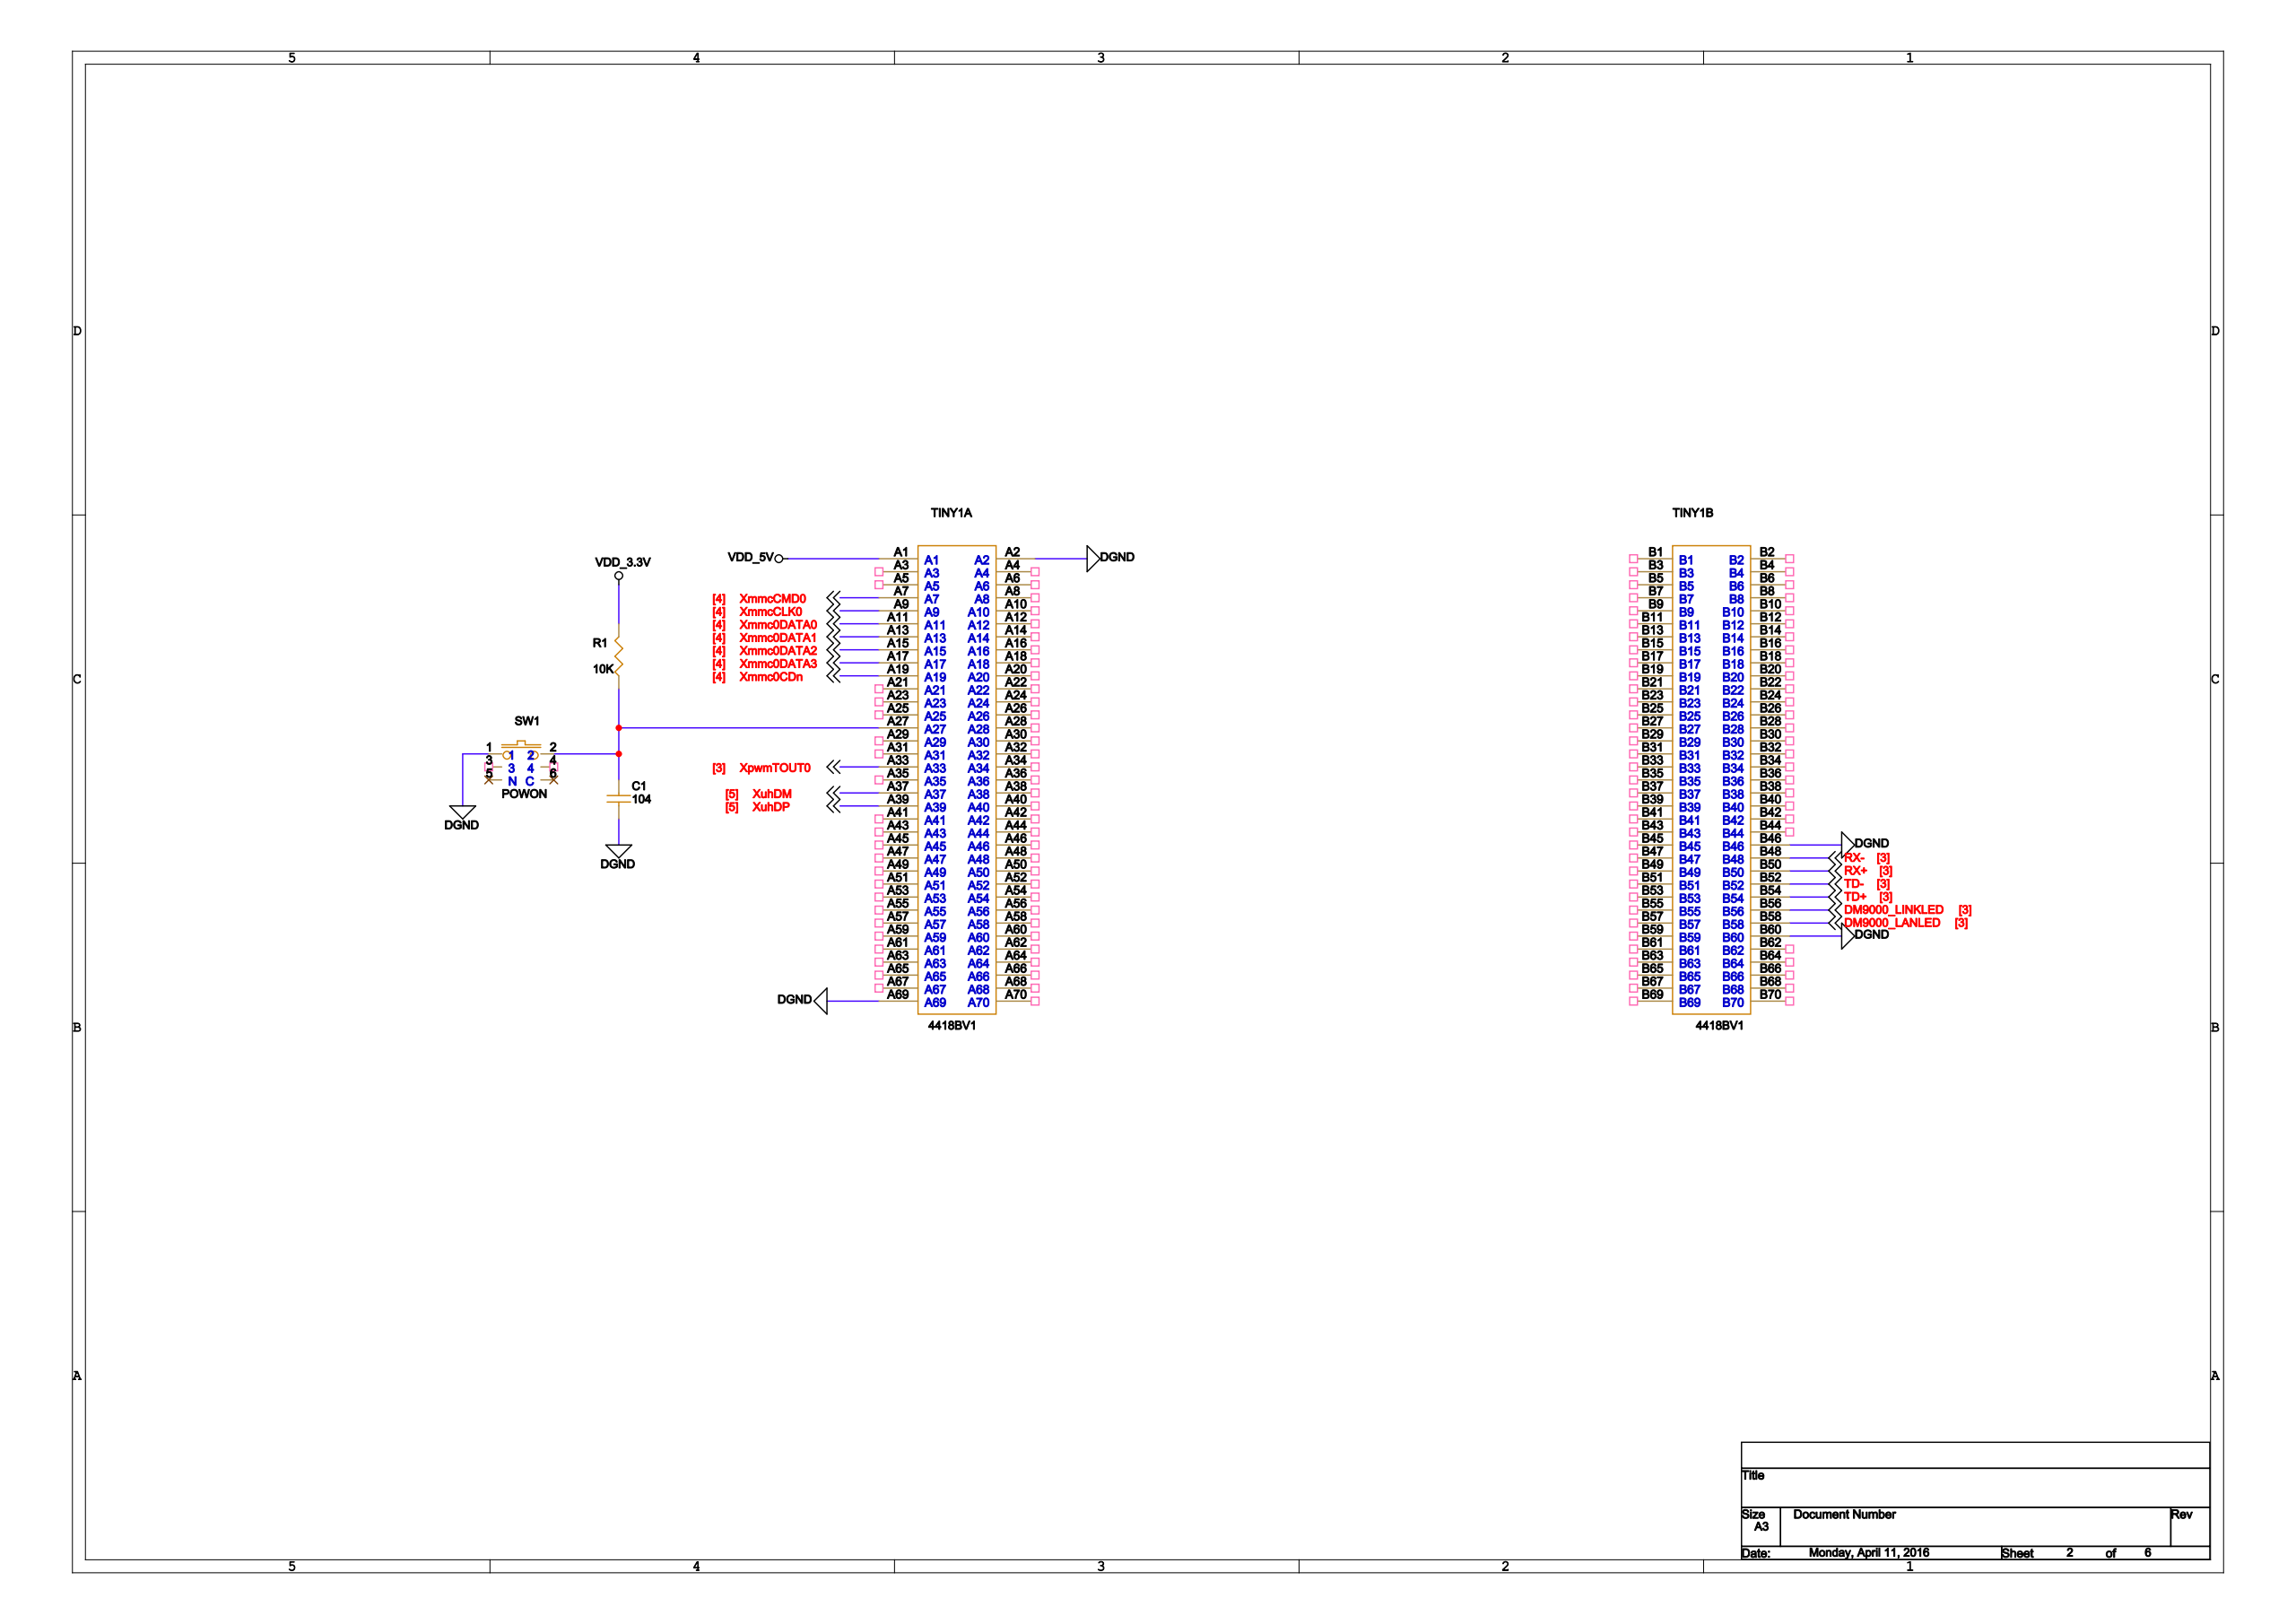Circuit board | Cadence Allegro | 85 parts | 48 nets | one sheet of the schematic
Parts on this sheet (reference | value | footprint):
C1 | 104 | C0603
R1 | 10K | R0603
SW1 | POWON | SMT_TD_15EA
TINY1 | 4418BV1 | TINYPRO
Nets of these parts (net: part-pin ...):
VDD_5V: TINY1-A1
DGND: C1-2 SW1-1 TINY1-A2 TINY1-A69 TINY1-B46 TINY1-B60
DM9000_LINKLED: TINY1-B56
DM9000_LANLED: TINY1-B58
RX+: TINY1-B50
RX-: TINY1-B48
TD+: TINY1-B54
TD-: TINY1-B52
VDD_3.3V: R1-2
N9814926: C1-1 R1-1 SW1-2 TINY1-A27